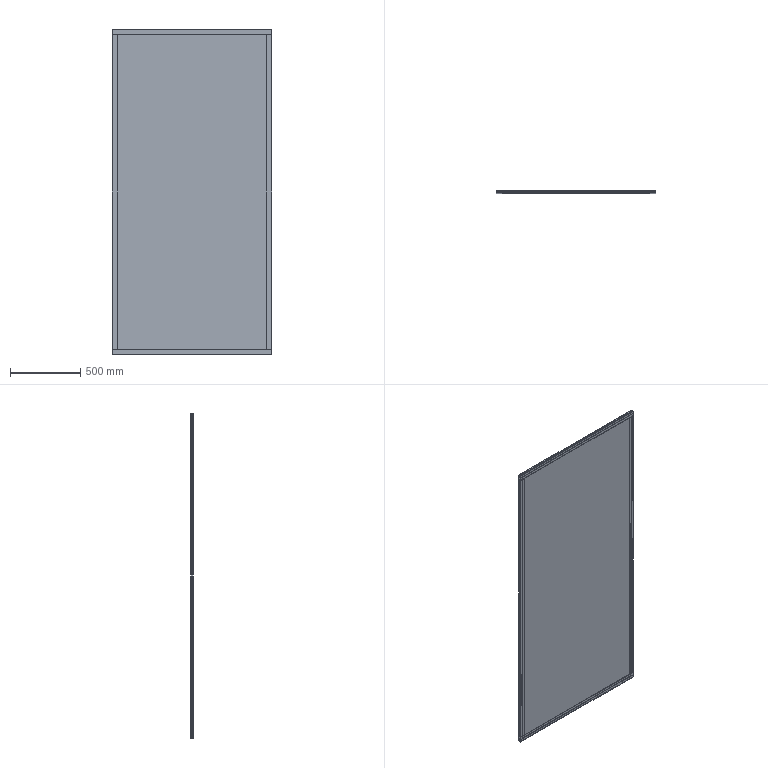Part | SolidWorks | 5 solids | 158 faces | box 1135 x 18 x 2317 mm | volume 26409670 mm3 | plane 94 | cylinder 64 | commonest cylinder face diameters 1.1 x24 3.6 x20 5.8 x20